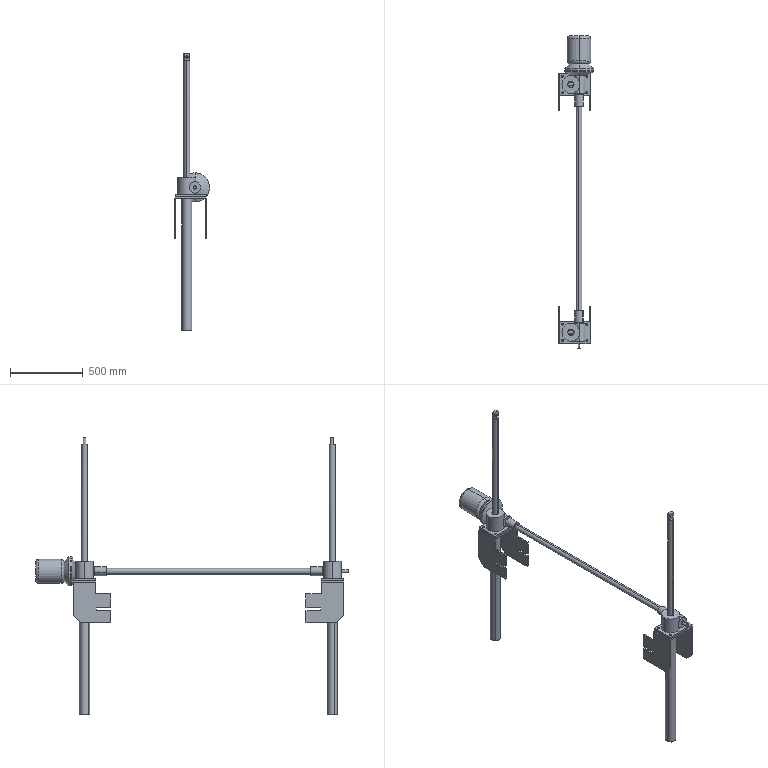Part | SolidWorks | features AEMSimFeature 1 | 25 solids | 362 faces | box 241 x 2141 x 1901 mm | volume 19247413 mm3 | cylinder 190 | plane 152 | cone 14 | torus 4 | spline 2 | commonest cylinder face diameters 40 x67 8 x19 12 x16 14 x16 20 x12 64 x8